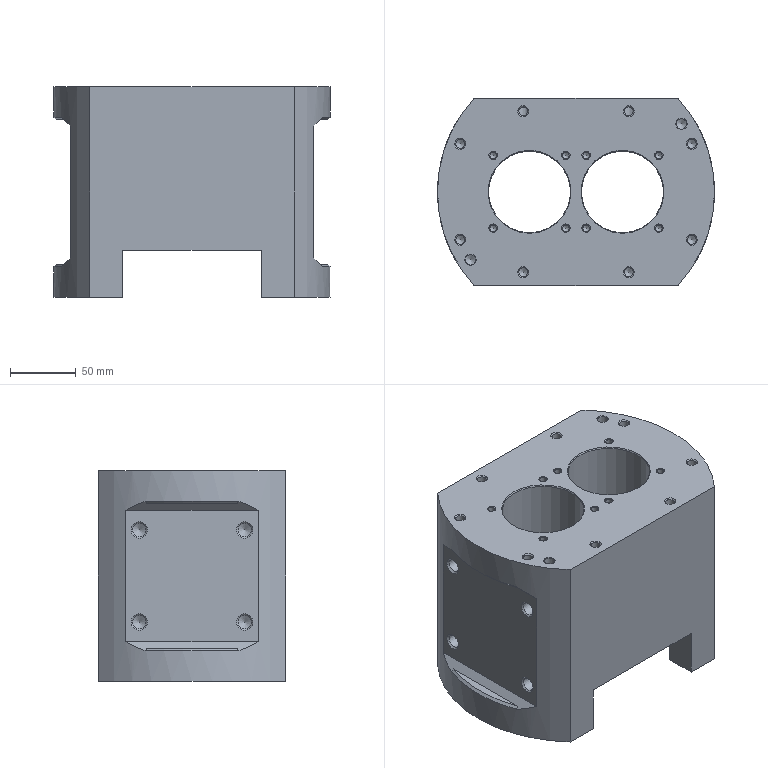NC program | NX | posted with a generic post | part box 210 x 142 x 160 mm
Lines 4710 to 4789 of 4789:
(DRILLING_COPY_1 , TOOL : ZXZ)
N9400 T01 M6
N9402 G54
N9404 G17 G0 G90 X-35. Y40. B0. C0. S5000 M3
N9406 G43 Z30. H1
N9408 G94 G81 G98 Z-13.75 F250. R-9.75
N9410 X35.
N9412 Y-40.
N9414 X-35.
N9416 G80
N9418 G0 X-35. Y-40. Z30.
N9420 M5
(DRILLING_COPY_COPY_1 , TOOL : 10.2ZT)
N9422 T11 M6
N9424 G54
N9426 G17 G0 G90 X-35. Y40. B0. C0. S1200 M3
N9428 G43 Z30. H11
N9430 G94 G83 G98 Z-41.814 F250. Q2. R-9.75
N9432 X35.
N9434 Y-40.
N9436 X-35.
N9438 G80
N9440 G0 X-35. Y-40. Z30.
N9442 M5
(PLANAR_MILL_COPY_COPY_COPY , TOOL : D6A45)
N9444 T07 M6
N9446 G54
N9448 G17 G0 G90 X-33.021 Y42.947 B0. C0. S7500 M3
N9450 G43 Z30. H7
N9452 Z-11.25
N9454 G94 G1 Z-14.25 F1250.
N9456 X-34.234 Y44.393
N9458 G3 X-35. Y44.75 R1.
N9460 X-39.75 Y40. R4.75
N9462 X-35. Y44.75 R-4.75
N9464 X-35.766 Y44.393 R1.
N9466 G1 X-36.979 Y42.947
N9468 Z-11.25
N9470 G0 Z30.
N9472 X36.979
N9474 Z-11.25
N9476 G1 Z-14.25
N9478 X35.766 Y44.393
N9480 G3 X35. Y44.75 R1.
N9482 X30.25 Y40. R4.75
N9484 X35. Y44.75 R-4.75
N9486 X34.234 Y44.393 R1.
N9488 G1 X33.021 Y42.947
N9490 Z-11.25
N9492 G0 Z30.
N9494 Y-42.947
N9496 Z-11.25
N9498 G1 Z-14.25
N9500 X34.234 Y-44.393
N9502 G3 X35. Y-44.75 R1.
N9504 X39.75 Y-40. R4.75
N9506 X35. Y-44.75 R-4.75
N9508 X35.766 Y-44.393 R1.
N9510 G1 X36.979 Y-42.947
N9512 Z-11.25
N9514 G0 Z30.
N9516 X-36.979
N9518 Z-11.25
N9520 G1 Z-14.25
N9522 X-35.766 Y-44.393
N9524 G3 X-35. Y-44.75 R1.
N9526 X-30.25 Y-40. R4.75
N9528 X-35. Y-44.75 R-4.75
N9530 X-34.234 Y-44.393 R1.
N9532 G1 X-33.021 Y-42.947
N9534 Z-11.25
N9536 G0 Z30.
N9538 M5
N9540 M2